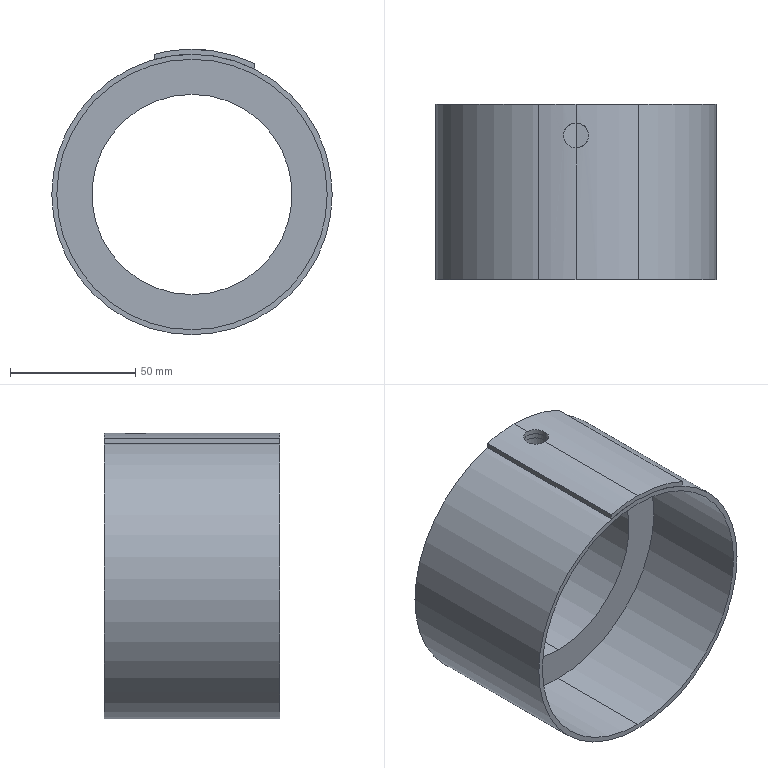Part | SolidWorks | features ICE 3, Extrusion 1 | 3 solids | 26 faces | box 112 x 70 x 114 mm | volume 156072 mm3 | cylinder 18 | plane 8 | commonest cylinder face diameters 10 x6 108 x4 112 x4 80 x2 116 x2
STEP:
#1=CARTESIAN_POINT('',(0.,7.5,54.));
#2=VERTEX_POINT('',#1);
#3=CARTESIAN_POINT('',(5.,12.5,53.768));
#4=VERTEX_POINT('',#3);
#5=CARTESIAN_POINT('',(0.,7.5,54.));
#6=CARTESIAN_POINT('',(0.3262,7.5,54.));
#7=CARTESIAN_POINT('',(0.6576,7.533,53.997));
#8=CARTESIAN_POINT('',(1.299,7.661,53.985));
#9=CARTESIAN_POINT('',(1.611,7.755,53.977));
#10=CARTESIAN_POINT('',(2.065,7.943,53.961));
#11=CARTESIAN_POINT('',(2.214,8.014,53.955));
#12=CARTESIAN_POINT('',(2.504,8.169,53.942));
#13=CARTESIAN_POINT('',(2.644,8.253,53.935));
#14=CARTESIAN_POINT('',(3.05,8.524,53.914));
#15=CARTESIAN_POINT('',(3.302,8.731,53.899));
#16=CARTESIAN_POINT('',(3.769,9.198,53.869));
#17=CARTESIAN_POINT('',(3.976,9.45,53.854));
#18=CARTESIAN_POINT('',(4.247,9.856,53.833));
#19=CARTESIAN_POINT('',(4.331,9.996,53.826));
#20=CARTESIAN_POINT('',(4.486,10.286,53.813));
#21=CARTESIAN_POINT('',(4.557,10.435,53.807));
#22=CARTESIAN_POINT('',(4.745,10.89,53.791));
#23=CARTESIAN_POINT('',(4.839,11.201,53.783));
#24=CARTESIAN_POINT('',(4.967,11.842,53.771));
#25=CARTESIAN_POINT('',(5.,12.174,53.768));
#26=CARTESIAN_POINT('',(5.,12.5,53.768));
#27=B_SPLINE_CURVE_WITH_KNOTS('',3,(#5,#6,#7,#8,#9,#10,#11,#12,#13,#14,#15,#16,#17,#18,#19,#20,#21,#22,#23,#24,#25,#26),.UNSPECIFIED.,.F.,.F.,(4,2,2,2,2,2,2,2,2,2,4),(0.007822,0.008799,0.009777,0.01027,0.01075,0.01173,0.01271,0.0132,0.01369,0.01466,0.01564),.UNSPECIFIED.);
#28=EDGE_CURVE('',#2,#4,#27,.T.);
#29=ORIENTED_EDGE('',*,*,#28,.T.);
#30=CARTESIAN_POINT('',(5.,12.5,39.686));
#31=VERTEX_POINT('',#30);
#32=CARTESIAN_POINT('',(5.,12.5,58.));
#33=DIRECTION('',(0.,0.,-1.));
#34=VECTOR('',#33,1000.);
#35=LINE('',#32,#34);
#36=EDGE_CURVE('',#4,#31,#35,.T.);
#37=ORIENTED_EDGE('',*,*,#36,.T.);
#38=CARTESIAN_POINT('',(0.,7.5,40.));
#39=VERTEX_POINT('',#38);
#40=CARTESIAN_POINT('',(0.,7.5,40.));
#41=CARTESIAN_POINT('',(0.3264,7.5,40.));
#42=CARTESIAN_POINT('',(0.658,7.533,39.996));
#43=CARTESIAN_POINT('',(1.299,7.661,39.98));
#44=CARTESIAN_POINT('',(1.611,7.755,39.969));
#45=CARTESIAN_POINT('',(2.065,7.944,39.947));
#46=CARTESIAN_POINT('',(2.215,8.014,39.939));
#47=CARTESIAN_POINT('',(2.504,8.169,39.922));
#48=CARTESIAN_POINT('',(2.644,8.253,39.913));
#49=CARTESIAN_POINT('',(3.05,8.525,39.884));
#50=CARTESIAN_POINT('',(3.303,8.732,39.864));
#51=CARTESIAN_POINT('',(3.769,9.198,39.823));
#52=CARTESIAN_POINT('',(3.976,9.45,39.802));
#53=CARTESIAN_POINT('',(4.247,9.856,39.774));
#54=CARTESIAN_POINT('',(4.331,9.996,39.765));
#55=CARTESIAN_POINT('',(4.486,10.285,39.748));
#56=CARTESIAN_POINT('',(4.557,10.435,39.74));
#57=CARTESIAN_POINT('',(4.745,10.889,39.718));
#58=CARTESIAN_POINT('',(4.839,11.201,39.706));
#59=CARTESIAN_POINT('',(4.967,11.842,39.69));
#60=CARTESIAN_POINT('',(5.,12.174,39.686));
#61=CARTESIAN_POINT('',(5.,12.5,39.686));
#62=B_SPLINE_CURVE_WITH_KNOTS('',3,(#40,#41,#42,#43,#44,#45,#46,#47,#48,#49,#50,#51,#52,#53,#54,#55,#56,#57,#58,#59,#60,#61),.UNSPECIFIED.,.F.,.F.,(4,2,2,2,2,2,2,2,2,2,4),(0.007826,0.008803,0.009781,0.01027,0.01076,0.01174,0.01271,0.0132,0.01369,0.01467,0.01565),.UNSPECIFIED.);
#63=EDGE_CURVE('',#39,#31,#62,.T.);
#64=ORIENTED_EDGE('',*,*,#63,.F.);
#65=CARTESIAN_POINT('',(-5.,12.5,39.686));
#66=VERTEX_POINT('',#65);
#67=CARTESIAN_POINT('',(-5.,12.5,39.686));
#68=CARTESIAN_POINT('',(-5.,12.169,39.686));
#69=CARTESIAN_POINT('',(-4.967,11.844,39.69));
#70=CARTESIAN_POINT('',(-4.872,11.364,39.702));
#71=CARTESIAN_POINT('',(-4.832,11.206,39.707));
#72=CARTESIAN_POINT('',(-4.737,10.891,39.719));
#73=CARTESIAN_POINT('',(-4.681,10.735,39.725));
#74=CARTESIAN_POINT('',(-4.493,10.281,39.747));
#75=CARTESIAN_POINT('',(-4.339,9.994,39.764));
#76=CARTESIAN_POINT('',(-3.976,9.45,39.802));
#77=CARTESIAN_POINT('',(-3.765,9.193,39.823));
#78=CARTESIAN_POINT('',(-3.304,8.733,39.864));
#79=CARTESIAN_POINT('',(-3.052,8.526,39.884));
#80=CARTESIAN_POINT('',(-2.505,8.16,39.922));
#81=CARTESIAN_POINT('',(-2.215,8.005,39.94));
#82=CARTESIAN_POINT('',(-1.613,7.756,39.969));
#83=CARTESIAN_POINT('',(-1.297,7.66,39.98));
#84=CARTESIAN_POINT('',(-0.6513,7.532,39.996));
#85=CARTESIAN_POINT('',(-0.3266,7.5,40.));
#86=CARTESIAN_POINT('',(0.,7.5,40.));
#87=B_SPLINE_CURVE_WITH_KNOTS('',3,(#67,#68,#69,#70,#71,#72,#73,#74,#75,#76,#77,#78,#79,#80,#81,#82,#83,#84,#85,#86),.UNSPECIFIED.,.F.,.F.,(4,2,2,2,2,2,2,2,2,4),(0.,0.0009782,0.001467,0.001956,0.002935,0.003913,0.004891,0.005869,0.006847,0.007826),.UNSPECIFIED.);
#88=EDGE_CURVE('',#66,#39,#87,.T.);
#89=ORIENTED_EDGE('',*,*,#88,.F.);
#90=CARTESIAN_POINT('',(-5.,12.5,53.768));
#91=VERTEX_POINT('',#90);
#92=CARTESIAN_POINT('',(-5.,12.5,58.));
#93=DIRECTION('',(0.,0.,-1.));
#94=VECTOR('',#93,1000.);
#95=LINE('',#92,#94);
#96=EDGE_CURVE('',#91,#66,#95,.T.);
#97=ORIENTED_EDGE('',*,*,#96,.F.);
#98=CARTESIAN_POINT('',(-5.,12.5,53.768));
#99=CARTESIAN_POINT('',(-5.,12.169,53.768));
#100=CARTESIAN_POINT('',(-4.968,11.844,53.771));
#101=CARTESIAN_POINT('',(-4.872,11.365,53.78));
#102=CARTESIAN_POINT('',(-4.832,11.206,53.783));
#103=CARTESIAN_POINT('',(-4.737,10.892,53.792));
#104=CARTESIAN_POINT('',(-4.681,10.736,53.797));
#105=CARTESIAN_POINT('',(-4.493,10.282,53.813));
#106=CARTESIAN_POINT('',(-4.339,9.994,53.826));
#107=CARTESIAN_POINT('',(-3.976,9.451,53.854));
#108=CARTESIAN_POINT('',(-3.765,9.194,53.869));
#109=CARTESIAN_POINT('',(-3.304,8.733,53.899));
#110=CARTESIAN_POINT('',(-3.052,8.526,53.914));
#111=CARTESIAN_POINT('',(-2.505,8.16,53.943));
#112=CARTESIAN_POINT('',(-2.214,8.005,53.955));
#113=CARTESIAN_POINT('',(-1.612,7.756,53.977));
#114=CARTESIAN_POINT('',(-1.297,7.66,53.985));
#115=CARTESIAN_POINT('',(-0.651,7.532,53.997));
#116=CARTESIAN_POINT('',(-0.3264,7.5,54.));
#117=CARTESIAN_POINT('',(0.,7.5,54.));
#118=B_SPLINE_CURVE_WITH_KNOTS('',3,(#98,#99,#100,#101,#102,#103,#104,#105,#106,#107,#108,#109,#110,#111,#112,#113,#114,#115,#116,#117),.UNSPECIFIED.,.F.,.F.,(4,2,2,2,2,2,2,2,2,4),(0.,0.0009778,0.001467,0.001956,0.002933,0.003911,0.004889,0.005867,0.006844,0.007822),.UNSPECIFIED.);
#119=EDGE_CURVE('',#91,#2,#118,.T.);
#120=ORIENTED_EDGE('',*,*,#119,.T.);
#121=EDGE_LOOP('',(#29,#37,#64,#89,#97,#120));
#122=FACE_OUTER_BOUND('',#121,.T.);
#123=CARTESIAN_POINT('',(0.,12.5,58.));
#124=DIRECTION('',(0.,0.,-1.));
#125=DIRECTION('',(-1.,0.,0.));
#126=AXIS2_PLACEMENT_3D('',#123,#124,#125);
#127=CYLINDRICAL_SURFACE('',#126,5.);
#128=ADVANCED_FACE('',(#122),#127,.F.);
#129=CARTESIAN_POINT('',(0.,25.,-40.));
#130=VERTEX_POINT('',#129);
#131=CARTESIAN_POINT('',(0.,25.,40.));
#132=VERTEX_POINT('',#131);
#133=CARTESIAN_POINT('',(0.,25.,0.));
#134=DIRECTION('',(0.,1.,0.));
#135=DIRECTION('',(0.,0.,1.));
#136=AXIS2_PLACEMENT_3D('',#133,#134,#135);
#137=CIRCLE('',#136,40.);
#138=EDGE_CURVE('',#130,#132,#137,.T.);
#139=ORIENTED_EDGE('',*,*,#138,.T.);
#140=CARTESIAN_POINT('',(0.,17.5,40.));
#141=VERTEX_POINT('',#140);
#142=CARTESIAN_POINT('',(0.,25.,40.));
#143=DIRECTION('',(0.,-1.,0.));
#144=VECTOR('',#143,1000.);
#145=LINE('',#142,#144);
#146=EDGE_CURVE('',#132,#141,#145,.T.);
#147=ORIENTED_EDGE('',*,*,#146,.T.);
#148=CARTESIAN_POINT('',(0.,17.5,40.));
#149=CARTESIAN_POINT('',(-0.3304,17.5,40.));
#150=CARTESIAN_POINT('',(-0.6553,17.468,39.996));
#151=CARTESIAN_POINT('',(-1.294,17.341,39.98));
#152=CARTESIAN_POINT('',(-1.612,17.244,39.969));
#153=CARTESIAN_POINT('',(-2.217,16.994,39.94));
#154=CARTESIAN_POINT('',(-2.504,16.84,39.922));
#155=CARTESIAN_POINT('',(-3.047,16.478,39.885));
#156=CARTESIAN_POINT('',(-3.304,16.267,39.864));
#157=CARTESIAN_POINT('',(-3.765,15.807,39.823));
#158=CARTESIAN_POINT('',(-3.972,15.555,39.803));
#159=CARTESIAN_POINT('',(-4.337,15.009,39.765));
#160=CARTESIAN_POINT('',(-4.492,14.719,39.747));
#161=CARTESIAN_POINT('',(-4.742,14.118,39.718));
#162=CARTESIAN_POINT('',(-4.838,13.803,39.706));
#163=CARTESIAN_POINT('',(-4.968,13.157,39.69));
#164=CARTESIAN_POINT('',(-5.,12.83,39.686));
#165=CARTESIAN_POINT('',(-5.,12.5,39.686));
#166=B_SPLINE_CURVE_WITH_KNOTS('',3,(#148,#149,#150,#151,#152,#153,#154,#155,#156,#157,#158,#159,#160,#161,#162,#163,#164,#165),.UNSPECIFIED.,.F.,.F.,(4,2,2,2,2,2,2,2,4),(0.02347,0.02445,0.02543,0.0264,0.02738,0.02836,0.02934,0.03031,0.03129),.UNSPECIFIED.);
#167=EDGE_CURVE('',#141,#66,#166,.T.);
#168=ORIENTED_EDGE('',*,*,#167,.T.);
#169=ORIENTED_EDGE('',*,*,#88,.T.);
#170=CARTESIAN_POINT('',(0.,0.,40.));
#171=VERTEX_POINT('',#170);
#172=CARTESIAN_POINT('',(0.,25.,40.));
#173=DIRECTION('',(0.,-1.,0.));
#174=VECTOR('',#173,1000.);
#175=LINE('',#172,#174);
#176=EDGE_CURVE('',#39,#171,#175,.T.);
#177=ORIENTED_EDGE('',*,*,#176,.T.);
#178=CARTESIAN_POINT('',(0.,0.,-40.));
#179=VERTEX_POINT('',#178);
#180=CARTESIAN_POINT('',(0.,0.,0.));
#181=DIRECTION('',(0.,1.,0.));
#182=DIRECTION('',(0.,0.,1.));
#183=AXIS2_PLACEMENT_3D('',#180,#181,#182);
#184=CIRCLE('',#183,40.);
#185=EDGE_CURVE('',#179,#171,#184,.T.);
#186=ORIENTED_EDGE('',*,*,#185,.F.);
#187=CARTESIAN_POINT('',(0.,25.,-40.));
#188=DIRECTION('',(0.,-1.,0.));
#189=VECTOR('',#188,1000.);
#190=LINE('',#187,#189);
#191=EDGE_CURVE('',#130,#179,#190,.T.);
#192=ORIENTED_EDGE('',*,*,#191,.F.);
#193=EDGE_LOOP('',(#139,#147,#168,#169,#177,#186,#192));
#194=FACE_OUTER_BOUND('',#193,.T.);
#195=CARTESIAN_POINT('',(0.,25.,0.));
#196=DIRECTION('',(0.,-1.,0.));
#197=DIRECTION('',(0.,0.,-1.));
#198=AXIS2_PLACEMENT_3D('',#195,#196,#197);
#199=CYLINDRICAL_SURFACE('',#198,40.);
#200=ADVANCED_FACE('',(#194),#199,.F.);
#201=CARTESIAN_POINT('',(0.,25.,54.));
#202=VERTEX_POINT('',#201);
#203=CARTESIAN_POINT('',(0.,25.,-54.));
#204=VERTEX_POINT('',#203);
#205=CARTESIAN_POINT('',(0.,25.,0.));
#206=DIRECTION('',(0.,1.,0.));
#207=DIRECTION('',(0.,0.,1.));
#208=AXIS2_PLACEMENT_3D('',#205,#206,#207);
#209=CIRCLE('',#208,54.);
#210=EDGE_CURVE('',#202,#204,#209,.T.);
#211=ORIENTED_EDGE('',*,*,#210,.F.);
#212=CARTESIAN_POINT('',(0.,17.5,54.));
#213=VERTEX_POINT('',#212);
#214=CARTESIAN_POINT('',(0.,25.,54.));
#215=DIRECTION('',(0.,-1.,0.));
#216=VECTOR('',#215,1000.);
#217=LINE('',#214,#216);
#218=EDGE_CURVE('',#202,#213,#217,.T.);
#219=ORIENTED_EDGE('',*,*,#218,.T.);
#220=CARTESIAN_POINT('',(5.,12.5,53.768));
#221=CARTESIAN_POINT('',(5.,12.826,53.768));
#222=CARTESIAN_POINT('',(4.968,13.151,53.771));
#223=CARTESIAN_POINT('',(4.84,13.796,53.783));
#224=CARTESIAN_POINT('',(4.744,14.112,53.791));
#225=CARTESIAN_POINT('',(4.495,14.714,53.813));
#226=CARTESIAN_POINT('',(4.34,15.005,53.826));
#227=CARTESIAN_POINT('',(3.974,15.552,53.854));
#228=CARTESIAN_POINT('',(3.767,15.804,53.869));
#229=CARTESIAN_POINT('',(3.306,16.265,53.899));
#230=CARTESIAN_POINT('',(3.049,16.476,53.915));
#231=CARTESIAN_POINT('',(2.505,16.839,53.943));
#232=CARTESIAN_POINT('',(2.218,16.993,53.955));
#233=CARTESIAN_POINT('',(1.764,17.181,53.971));
#234=CARTESIAN_POINT('',(1.608,17.237,53.976));
#235=CARTESIAN_POINT('',(1.294,17.333,53.985));
#236=CARTESIAN_POINT('',(1.135,17.372,53.988));
#237=CARTESIAN_POINT('',(0.6554,17.468,53.997));
#238=CARTESIAN_POINT('',(0.3304,17.5,54.));
#239=CARTESIAN_POINT('',(0.,17.5,54.));
#240=B_SPLINE_CURVE_WITH_KNOTS('',3,(#220,#221,#222,#223,#224,#225,#226,#227,#228,#229,#230,#231,#232,#233,#234,#235,#236,#237,#238,#239),.UNSPECIFIED.,.F.,.F.,(4,2,2,2,2,2,2,2,2,4),(0.01564,0.01662,0.0176,0.01857,0.01955,0.02053,0.02151,0.022,0.02249,0.02346),.UNSPECIFIED.);
#241=EDGE_CURVE('',#4,#213,#240,.T.);
#242=ORIENTED_EDGE('',*,*,#241,.F.);
#243=ORIENTED_EDGE('',*,*,#28,.F.);
#244=CARTESIAN_POINT('',(0.,0.,54.));
#245=VERTEX_POINT('',#244);
#246=CARTESIAN_POINT('',(0.,25.,54.));
#247=DIRECTION('',(0.,-1.,0.));
#248=VECTOR('',#247,1000.);
#249=LINE('',#246,#248);
#250=EDGE_CURVE('',#2,#245,#249,.T.);
#251=ORIENTED_EDGE('',*,*,#250,.T.);
#252=CARTESIAN_POINT('',(0.,0.,-54.));
#253=VERTEX_POINT('',#252);
#254=CARTESIAN_POINT('',(0.,0.,0.));
#255=DIRECTION('',(0.,1.,0.));
#256=DIRECTION('',(0.,0.,1.));
#257=AXIS2_PLACEMENT_3D('',#254,#255,#256);
#258=CIRCLE('',#257,54.);
#259=EDGE_CURVE('',#245,#253,#258,.T.);
#260=ORIENTED_EDGE('',*,*,#259,.T.);
#261=CARTESIAN_POINT('',(0.,25.,-54.));
#262=DIRECTION('',(0.,-1.,0.));
#263=VECTOR('',#262,1000.);
#264=LINE('',#261,#263);
#265=EDGE_CURVE('',#204,#253,#264,.T.);
#266=ORIENTED_EDGE('',*,*,#265,.F.);
#267=EDGE_LOOP('',(#211,#219,#242,#243,#251,#260,#266));
#268=FACE_OUTER_BOUND('',#267,.T.);
#269=CARTESIAN_POINT('',(0.,25.,0.));
#270=DIRECTION('',(0.,-1.,0.));
#271=DIRECTION('',(0.,0.,-1.));
#272=AXIS2_PLACEMENT_3D('',#269,#270,#271);
#273=CYLINDRICAL_SURFACE('',#272,54.);
#274=ADVANCED_FACE('',(#268),#273,.T.);
#275=ORIENTED_EDGE('',*,*,#218,.F.);
#276=CARTESIAN_POINT('',(0.,25.,0.));
#277=DIRECTION('',(0.,1.,0.));
#278=DIRECTION('',(0.,0.,1.));
#279=AXIS2_PLACEMENT_3D('',#276,#277,#278);
#280=CIRCLE('',#279,54.);
#281=EDGE_CURVE('',#204,#202,#280,.T.);
#282=ORIENTED_EDGE('',*,*,#281,.F.);
#283=ORIENTED_EDGE('',*,*,#265,.T.);
#284=CARTESIAN_POINT('',(0.,0.,0.));
#285=DIRECTION('',(0.,1.,0.));
#286=DIRECTION('',(0.,0.,1.));
#287=AXIS2_PLACEMENT_3D('',#284,#285,#286);
#288=CIRCLE('',#287,54.);
#289=EDGE_CURVE('',#253,#245,#288,.T.);
#290=ORIENTED_EDGE('',*,*,#289,.T.);
#291=ORIENTED_EDGE('',*,*,#250,.F.);
#292=ORIENTED_EDGE('',*,*,#119,.F.);
#293=CARTESIAN_POINT('',(0.,17.5,54.));
#294=CARTESIAN_POINT('',(-0.3301,17.5,54.));
#295=CARTESIAN_POINT('',(-0.6554,17.468,53.997));
#296=CARTESIAN_POINT('',(-1.135,17.372,53.988));
#297=CARTESIAN_POINT('',(-1.293,17.333,53.985));
#298=CARTESIAN_POINT('',(-1.607,17.238,53.976));
#299=CARTESIAN_POINT('',(-1.763,17.182,53.971));
#300=CARTESIAN_POINT('',(-2.217,16.994,53.955));
#301=CARTESIAN_POINT('',(-2.504,16.84,53.943));
#302=CARTESIAN_POINT('',(-3.047,16.478,53.915));
#303=CARTESIAN_POINT('',(-3.304,16.267,53.899));
#304=CARTESIAN_POINT('',(-3.765,15.806,53.869));
#305=CARTESIAN_POINT('',(-3.972,15.555,53.854));
#306=CARTESIAN_POINT('',(-4.337,15.009,53.826));
#307=CARTESIAN_POINT('',(-4.493,14.719,53.813));
#308=CARTESIAN_POINT('',(-4.742,14.117,53.792));
#309=CARTESIAN_POINT('',(-4.838,13.803,53.783));
#310=CARTESIAN_POINT('',(-4.968,13.157,53.771));
#311=CARTESIAN_POINT('',(-5.,12.83,53.768));
#312=CARTESIAN_POINT('',(-5.,12.5,53.768));
#313=B_SPLINE_CURVE_WITH_KNOTS('',3,(#293,#294,#295,#296,#297,#298,#299,#300,#301,#302,#303,#304,#305,#306,#307,#308,#309,#310,#311,#312),.UNSPECIFIED.,.F.,.F.,(4,2,2,2,2,2,2,2,2,4),(0.02346,0.02444,0.02493,0.02542,0.02639,0.02737,0.02835,0.02932,0.0303,0.03128),.UNSPECIFIED.);
#314=EDGE_CURVE('',#213,#91,#313,.T.);
#315=ORIENTED_EDGE('',*,*,#314,.F.);
#316=EDGE_LOOP('',(#275,#282,#283,#290,#291,#292,#315));
#317=FACE_OUTER_BOUND('',#316,.T.);
#318=CARTESIAN_POINT('',(0.,25.,0.));
#319=DIRECTION('',(0.,-1.,0.));
#320=DIRECTION('',(0.,0.,-1.));
#321=AXIS2_PLACEMENT_3D('',#318,#319,#320);
#322=CYLINDRICAL_SURFACE('',#321,54.);
#323=ADVANCED_FACE('',(#317),#322,.T.);
#324=ORIENTED_EDGE('',*,*,#146,.F.);
#325=CARTESIAN_POINT('',(0.,25.,0.));
#326=DIRECTION('',(0.,1.,0.));
#327=DIRECTION('',(0.,0.,1.));
#328=AXIS2_PLACEMENT_3D('',#325,#326,#327);
#329=CIRCLE('',#328,40.);
#330=EDGE_CURVE('',#132,#130,#329,.T.);
#331=ORIENTED_EDGE('',*,*,#330,.T.);
#332=ORIENTED_EDGE('',*,*,#191,.T.);
#333=CARTESIAN_POINT('',(0.,0.,0.));
#334=DIRECTION('',(0.,1.,0.));
#335=DIRECTION('',(0.,0.,1.));
#336=AXIS2_PLACEMENT_3D('',#333,#334,#335);
#337=CIRCLE('',#336,40.);
#338=EDGE_CURVE('',#171,#179,#337,.T.);
#339=ORIENTED_EDGE('',*,*,#338,.F.);
#340=ORIENTED_EDGE('',*,*,#176,.F.);
#341=ORIENTED_EDGE('',*,*,#63,.T.);
#342=CARTESIAN_POINT('',(5.,12.5,39.686));
#343=CARTESIAN_POINT('',(5.,12.827,39.686));
#344=CARTESIAN_POINT('',(4.968,13.151,39.69));
#345=CARTESIAN_POINT('',(4.84,13.797,39.706));
#346=CARTESIAN_POINT('',(4.744,14.113,39.718));
#347=CARTESIAN_POINT('',(4.495,14.715,39.747));
#348=CARTESIAN_POINT('',(4.339,15.006,39.764));
#349=CARTESIAN_POINT('',(3.974,15.552,39.803));
#350=CARTESIAN_POINT('',(3.767,15.804,39.823));
#351=CARTESIAN_POINT('',(3.306,16.265,39.864));
#352=CARTESIAN_POINT('',(3.049,16.476,39.885));
#353=CARTESIAN_POINT('',(2.506,16.839,39.922));
#354=CARTESIAN_POINT('',(2.219,16.993,39.94));
#355=CARTESIAN_POINT('',(1.765,17.181,39.961));
#356=CARTESIAN_POINT('',(1.608,17.237,39.968));
#357=CARTESIAN_POINT('',(1.294,17.332,39.979));
#358=CARTESIAN_POINT('',(1.136,17.372,39.984));
#359=CARTESIAN_POINT('',(0.6561,17.467,39.996));
#360=CARTESIAN_POINT('',(0.3307,17.5,40.));
#361=CARTESIAN_POINT('',(0.,17.5,40.));
#362=B_SPLINE_CURVE_WITH_KNOTS('',3,(#342,#343,#344,#345,#346,#347,#348,#349,#350,#351,#352,#353,#354,#355,#356,#357,#358,#359,#360,#361),.UNSPECIFIED.,.F.,.F.,(4,2,2,2,2,2,2,2,2,4),(0.01565,0.01663,0.0176,0.01858,0.01956,0.02054,0.02152,0.02201,0.02249,0.02347),.UNSPECIFIED.);
#363=EDGE_CURVE('',#31,#141,#362,.T.);
#364=ORIENTED_EDGE('',*,*,#363,.T.);
#365=EDGE_LOOP('',(#324,#331,#332,#339,#340,#341,#364));
#366=FACE_OUTER_BOUND('',#365,.T.);
#367=CARTESIAN_POINT('',(0.,25.,0.));
#368=DIRECTION('',(0.,-1.,0.));
#369=DIRECTION('',(0.,0.,-1.));
#370=AXIS2_PLACEMENT_3D('',#367,#368,#369);
#371=CYLINDRICAL_SURFACE('',#370,40.);
#372=ADVANCED_FACE('',(#366),#371,.F.);
#373=ORIENTED_EDGE('',*,*,#281,.T.);
#374=ORIENTED_EDGE('',*,*,#210,.T.);
#375=EDGE_LOOP('',(#373,#374));
#376=FACE_OUTER_BOUND('',#375,.T.);
#377=ORIENTED_EDGE('',*,*,#138,.F.);
#378=ORIENTED_EDGE('',*,*,#330,.F.);
#379=EDGE_LOOP('',(#377,#378));
#380=FACE_BOUND('',#379,.T.);
#381=CARTESIAN_POINT('',(0.,25.,0.));
#382=DIRECTION('',(0.,1.,0.));
#383=DIRECTION('',(0.,0.,1.));
#384=AXIS2_PLACEMENT_3D('',#381,#382,#383);
#385=PLANE('',#384);
#386=ADVANCED_FACE('',(#376,#380),#385,.T.);
#387=ORIENTED_EDGE('',*,*,#289,.F.);
#388=ORIENTED_EDGE('',*,*,#259,.F.);
#389=EDGE_LOOP('',(#387,#388));
#390=FACE_OUTER_BOUND('',#389,.T.);
#391=ORIENTED_EDGE('',*,*,#185,.T.);
#392=ORIENTED_EDGE('',*,*,#338,.T.);
#393=EDGE_LOOP('',(#391,#392));
#394=FACE_BOUND('',#393,.T.);
#395=CARTESIAN_POINT('',(0.,0.,0.));
#396=DIRECTION('',(0.,1.,0.));
#397=DIRECTION('',(0.,0.,1.));
#398=AXIS2_PLACEMENT_3D('',#395,#396,#397);
#399=PLANE('',#398);
#400=ADVANCED_FACE('',(#390,#394),#399,.F.);
#401=ORIENTED_EDGE('',*,*,#36,.F.);
#402=ORIENTED_EDGE('',*,*,#241,.T.);
#403=ORIENTED_EDGE('',*,*,#314,.T.);
#404=ORIENTED_EDGE('',*,*,#96,.T.);
#405=ORIENTED_EDGE('',*,*,#167,.F.);
#406=ORIENTED_EDGE('',*,*,#363,.F.);
#407=EDGE_LOOP('',(#401,#402,#403,#404,#405,#406));
#408=FACE_OUTER_BOUND('',#407,.T.);
#409=CARTESIAN_POINT('',(0.,12.5,58.));
#410=DIRECTION('',(0.,0.,-1.));
#411=DIRECTION('',(-1.,0.,0.));
#412=AXIS2_PLACEMENT_3D('',#409,#410,#411);
#413=CYLINDRICAL_SURFACE('',#412,5.);
#414=ADVANCED_FACE('',(#408),#413,.F.);
#415=CLOSED_SHELL('',(#128,#200,#274,#323,#372,#386,#400,#414));
#416=MANIFOLD_SOLID_BREP('',#415);
#417=CARTESIAN_POINT('',(5.,12.5,55.776));
#418=VERTEX_POINT('',#417);
#419=CARTESIAN_POINT('',(0.,7.5,56.));
#420=VERTEX_POINT('',#419);
#421=CARTESIAN_POINT('',(5.,12.5,55.776));
#422=CARTESIAN_POINT('',(5.,12.17,55.776));
#423=CARTESIAN_POINT('',(4.968,11.845,55.779));
#424=CARTESIAN_POINT('',(4.872,11.366,55.788));
#425=CARTESIAN_POINT('',(4.833,11.207,55.791));
#426=CARTESIAN_POINT('',(4.738,10.893,55.799));
#427=CARTESIAN_POINT('',(4.682,10.737,55.804));
#428=CARTESIAN_POINT('',(4.494,10.283,55.82));
#429=CARTESIAN_POINT('',(4.34,9.996,55.832));
#430=CARTESIAN_POINT('',(3.978,9.453,55.859));
#431=CARTESIAN_POINT('',(3.767,9.196,55.874));
#432=CARTESIAN_POINT('',(3.306,8.735,55.903));
#433=CARTESIAN_POINT('',(3.055,8.528,55.917));
#434=CARTESIAN_POINT('',(2.509,8.163,55.944));
#435=CARTESIAN_POINT('',(2.218,8.007,55.957));
#436=CARTESIAN_POINT('',(1.617,7.758,55.977));
#437=CARTESIAN_POINT('',(1.303,7.662,55.986));
#438=CARTESIAN_POINT('',(0.657,7.532,55.997));
#439=CARTESIAN_POINT('',(0.3303,7.5,56.));
#440=CARTESIAN_POINT('',(0.,7.5,56.));
#441=B_SPLINE_CURVE_WITH_KNOTS('',3,(#421,#422,#423,#424,#425,#426,#427,#428,#429,#430,#431,#432,#433,#434,#435,#436,#437,#438,#439,#440),.UNSPECIFIED.,.F.,.F.,(4,2,2,2,2,2,2,2,2,4),(0.02346,0.02444,0.02493,0.02542,0.02639,0.02737,0.02835,0.02932,0.0303,0.03128),.UNSPECIFIED.);
#442=EDGE_CURVE('',#418,#420,#441,.T.);
#443=ORIENTED_EDGE('',*,*,#442,.F.);
#444=CARTESIAN_POINT('',(5.,12.5,53.768));
#445=VERTEX_POINT('',#444);
#446=CARTESIAN_POINT('',(5.,12.5,58.));
#447=DIRECTION('',(0.,0.,-1.));
#448=VECTOR('',#447,1000.);
#449=LINE('',#446,#448);
#450=EDGE_CURVE('',#418,#445,#449,.T.);
#451=ORIENTED_EDGE('',*,*,#450,.T.);
#452=CARTESIAN_POINT('',(0.,7.5,54.));
#453=VERTEX_POINT('',#452);
#454=CARTESIAN_POINT('',(5.,12.5,53.768));
#455=CARTESIAN_POINT('',(5.,12.17,53.768));
#456=CARTESIAN_POINT('',(4.968,11.845,53.771));
#457=CARTESIAN_POINT('',(4.872,11.365,53.78));
#458=CARTESIAN_POINT('',(4.833,11.207,53.783));
#459=CARTESIAN_POINT('',(4.738,10.893,53.792));
#460=CARTESIAN_POINT('',(4.682,10.737,53.797));
#461=CARTESIAN_POINT('',(4.494,10.283,53.813));
#462=CARTESIAN_POINT('',(4.34,9.996,53.826));
#463=CARTESIAN_POINT('',(3.978,9.453,53.854));
#464=CARTESIAN_POINT('',(3.767,9.196,53.869));
#465=CARTESIAN_POINT('',(3.306,8.735,53.899));
#466=CARTESIAN_POINT('',(3.055,8.528,53.914));
#467=CARTESIAN_POINT('',(2.509,8.163,53.942));
#468=CARTESIAN_POINT('',(2.219,8.007,53.955));
#469=CARTESIAN_POINT('',(1.617,7.758,53.977));
#470=CARTESIAN_POINT('',(1.303,7.662,53.985));
#471=CARTESIAN_POINT('',(0.657,7.532,53.997));
#472=CARTESIAN_POINT('',(0.3303,7.5,54.));
#473=CARTESIAN_POINT('',(0.,7.5,54.));
#474=B_SPLINE_CURVE_WITH_KNOTS('',3,(#454,#455,#456,#457,#458,#459,#460,#461,#462,#463,#464,#465,#466,#467,#468,#469,#470,#471,#472,#473),.UNSPECIFIED.,.F.,.F.,(4,2,2,2,2,2,2,2,2,4),(0.02346,0.02444,0.02493,0.02542,0.02639,0.02737,0.02835,0.02932,0.0303,0.03128),.UNSPECIFIED.);
#475=EDGE_CURVE('',#445,#453,#474,.T.);
#476=ORIENTED_EDGE('',*,*,#475,.T.);
#477=CARTESIAN_POINT('',(-5.,12.5,53.768));
#478=VERTEX_POINT('',#477);
#479=CARTESIAN_POINT('',(0.,7.5,54.));
#480=CARTESIAN_POINT('',(-0.3306,7.5,54.));
#481=CARTESIAN_POINT('',(-0.6557,7.532,53.997));
#482=CARTESIAN_POINT('',(-1.135,7.628,53.988));
#483=CARTESIAN_POINT('',(-1.294,7.668,53.985));
#484=CARTESIAN_POINT('',(-1.608,7.763,53.976));
#485=CARTESIAN_POINT('',(-1.764,7.819,53.971));
#486=CARTESIAN_POINT('',(-2.218,8.007,53.955));
#487=CARTESIAN_POINT('',(-2.506,8.161,53.943));
#488=CARTESIAN_POINT('',(-3.049,8.524,53.915));
#489=CARTESIAN_POINT('',(-3.306,8.735,53.899));
#490=CARTESIAN_POINT('',(-3.767,9.196,53.869));
#491=CARTESIAN_POINT('',(-3.974,9.448,53.854));
#492=CARTESIAN_POINT('',(-4.34,9.995,53.826));
#493=CARTESIAN_POINT('',(-4.495,10.286,53.813));
#494=CARTESIAN_POINT('',(-4.744,10.888,53.791));
#495=CARTESIAN_POINT('',(-4.84,11.203,53.783));
#496=CARTESIAN_POINT('',(-4.968,11.849,53.771));
#497=CARTESIAN_POINT('',(-5.,12.174,53.768));
#498=CARTESIAN_POINT('',(-5.,12.5,53.768));
#499=B_SPLINE_CURVE_WITH_KNOTS('',3,(#479,#480,#481,#482,#483,#484,#485,#486,#487,#488,#489,#490,#491,#492,#493,#494,#495,#496,#497,#498),.UNSPECIFIED.,.F.,.F.,(4,2,2,2,2,2,2,2,2,4),(0.,0.0009778,0.001467,0.001956,0.002933,0.003911,0.004889,0.005867,0.006844,0.007822),.UNSPECIFIED.);
#500=EDGE_CURVE('',#453,#478,#499,.T.);
#501=ORIENTED_EDGE('',*,*,#500,.T.);
#502=CARTESIAN_POINT('',(-5.,12.5,55.776));
#503=VERTEX_POINT('',#502);
#504=CARTESIAN_POINT('',(-5.,12.5,58.));
#505=DIRECTION('',(0.,0.,-1.));
#506=VECTOR('',#505,1000.);
#507=LINE('',#504,#506);
#508=EDGE_CURVE('',#503,#478,#507,.T.);
#509=ORIENTED_EDGE('',*,*,#508,.F.);
#510=CARTESIAN_POINT('',(0.,7.5,56.));
#511=CARTESIAN_POINT('',(-0.3306,7.5,56.));
#512=CARTESIAN_POINT('',(-0.6557,7.532,55.997));
#513=CARTESIAN_POINT('',(-1.135,7.628,55.989));
#514=CARTESIAN_POINT('',(-1.294,7.667,55.985));
#515=CARTESIAN_POINT('',(-1.608,7.763,55.977));
#516=CARTESIAN_POINT('',(-1.764,7.819,55.972));
#517=CARTESIAN_POINT('',(-2.218,8.007,55.957));
#518=CARTESIAN_POINT('',(-2.506,8.161,55.945));
#519=CARTESIAN_POINT('',(-3.049,8.524,55.918));
#520=CARTESIAN_POINT('',(-3.306,8.735,55.903));
#521=CARTESIAN_POINT('',(-3.767,9.196,55.874));
#522=CARTESIAN_POINT('',(-3.974,9.448,55.859));
#523=CARTESIAN_POINT('',(-4.34,9.995,55.832));
#524=CARTESIAN_POINT('',(-4.495,10.286,55.819));
#525=CARTESIAN_POINT('',(-4.744,10.888,55.799));
#526=CARTESIAN_POINT('',(-4.84,11.203,55.79));
#527=CARTESIAN_POINT('',(-4.968,11.849,55.779));
#528=CARTESIAN_POINT('',(-5.,12.174,55.776));
#529=CARTESIAN_POINT('',(-5.,12.5,55.776));
#530=B_SPLINE_CURVE_WITH_KNOTS('',3,(#510,#511,#512,#513,#514,#515,#516,#517,#518,#519,#520,#521,#522,#523,#524,#525,#526,#527,#528,#529),.UNSPECIFIED.,.F.,.F.,(4,2,2,2,2,2,2,2,2,4),(0.,0.0009777,0.001467,0.001955,0.002933,0.003911,0.004889,0.005866,0.006844,0.007822),.UNSPECIFIED.);
#531=EDGE_CURVE('',#420,#503,#530,.T.);
#532=ORIENTED_EDGE('',*,*,#531,.F.);
#533=EDGE_LOOP('',(#443,#451,#476,#501,#509,#532));
#534=FACE_OUTER_BOUND('',#533,.T.);
#535=CARTESIAN_POINT('',(0.,12.5,58.));
#536=DIRECTION('',(0.,0.,-1.));
#537=DIRECTION('',(-1.,0.,0.));
#538=AXIS2_PLACEMENT_3D('',#535,#536,#537);
#539=CYLINDRICAL_SURFACE('',#538,5.);
#540=ADVANCED_FACE('',(#534),#539,.F.);
#541=CARTESIAN_POINT('',(0.,-45.,-54.));
#542=VERTEX_POINT('',#541);
#543=CARTESIAN_POINT('',(0.,-45.,54.));
#544=VERTEX_POINT('',#543);
#545=CARTESIAN_POINT('',(0.,-45.,0.));
#546=DIRECTION('',(0.,1.,0.));
#547=DIRECTION('',(0.,0.,1.));
#548=AXIS2_PLACEMENT_3D('',#545,#546,#547);
#549=CIRCLE('',#548,54.);
#550=EDGE_CURVE('',#542,#544,#549,.T.);
#551=ORIENTED_EDGE('',*,*,#550,.F.);
#552=CARTESIAN_POINT('',(0.,25.,-54.));
#553=VERTEX_POINT('',#552);
#554=CARTESIAN_POINT('',(0.,-45.,-54.));
#555=DIRECTION('',(0.,1.,0.));
#556=VECTOR('',#555,1000.);
#557=LINE('',#554,#556);
#558=EDGE_CURVE('',#542,#553,#557,.T.);
#559=ORIENTED_EDGE('',*,*,#558,.T.);
#560=CARTESIAN_POINT('',(0.,25.,54.));
#561=VERTEX_POINT('',#560);
#562=CARTESIAN_POINT('',(0.,25.,0.));
#563=DIRECTION('',(0.,1.,0.));
#564=DIRECTION('',(0.,0.,1.));
#565=AXIS2_PLACEMENT_3D('',#562,#563,#564);
#566=CIRCLE('',#565,54.);
#567=EDGE_CURVE('',#553,#561,#566,.T.);
#568=ORIENTED_EDGE('',*,*,#567,.T.);
#569=CARTESIAN_POINT('',(0.,17.5,54.));
#570=VERTEX_POINT('',#569);
#571=CARTESIAN_POINT('',(0.,-45.,54.));
#572=DIRECTION('',(0.,1.,0.));
#573=VECTOR('',#572,1000.);
#574=LINE('',#571,#573);
#575=EDGE_CURVE('',#570,#561,#574,.T.);
#576=ORIENTED_EDGE('',*,*,#575,.F.);
#577=CARTESIAN_POINT('',(-5.,12.5,53.768));
#578=CARTESIAN_POINT('',(-5.,12.826,53.768));
#579=CARTESIAN_POINT('',(-4.967,13.158,53.771));
#580=CARTESIAN_POINT('',(-4.839,13.799,53.783));
#581=CARTESIAN_POINT('',(-4.745,14.111,53.791));
#582=CARTESIAN_POINT('',(-4.557,14.565,53.807));
#583=CARTESIAN_POINT('',(-4.486,14.714,53.813));
#584=CARTESIAN_POINT('',(-4.331,15.004,53.826));
#585=CARTESIAN_POINT('',(-4.247,15.144,53.833));
#586=CARTESIAN_POINT('',(-3.976,15.55,53.854));
#587=CARTESIAN_POINT('',(-3.769,15.802,53.869));
#588=CARTESIAN_POINT('',(-3.302,16.269,53.899));
#589=CARTESIAN_POINT('',(-3.05,16.476,53.915));
#590=CARTESIAN_POINT('',(-2.644,16.747,53.935));
#591=CARTESIAN_POINT('',(-2.504,16.831,53.942));
#592=CARTESIAN_POINT('',(-2.214,16.986,53.955));
#593=CARTESIAN_POINT('',(-2.065,17.057,53.961));
#594=CARTESIAN_POINT('',(-1.61,17.245,53.977));
#595=CARTESIAN_POINT('',(-1.299,17.339,53.985));
#596=CARTESIAN_POINT('',(-0.6578,17.467,53.997));
#597=CARTESIAN_POINT('',(-0.3263,17.5,54.));
#598=CARTESIAN_POINT('',(0.,17.5,54.));
#599=B_SPLINE_CURVE_WITH_KNOTS('',3,(#577,#578,#579,#580,#581,#582,#583,#584,#585,#586,#587,#588,#589,#590,#591,#592,#593,#594,#595,#596,#597,#598),.UNSPECIFIED.,.F.,.F.,(4,2,2,2,2,2,2,2,2,2,4),(0.007822,0.008799,0.009777,0.01027,0.01075,0.01173,0.01271,0.0132,0.01369,0.01466,0.01564),.UNSPECIFIED.);
#600=EDGE_CURVE('',#478,#570,#599,.T.);
#601=ORIENTED_EDGE('',*,*,#600,.F.);
#602=ORIENTED_EDGE('',*,*,#500,.F.);
#603=CARTESIAN_POINT('',(0.,-45.,54.));
#604=DIRECTION('',(0.,1.,0.));
#605=VECTOR('',#604,1000.);
#606=LINE('',#603,#605);
#607=EDGE_CURVE('',#544,#453,#606,.T.);
#608=ORIENTED_EDGE('',*,*,#607,.F.);
#609=EDGE_LOOP('',(#551,#559,#568,#576,#601,#602,#608));
#610=FACE_OUTER_BOUND('',#609,.T.);
#611=CARTESIAN_POINT('',(0.,-45.,0.));
#612=DIRECTION('',(0.,1.,0.));
#613=DIRECTION('',(0.,0.,1.));
#614=AXIS2_PLACEMENT_3D('',#611,#612,#613);
#615=CYLINDRICAL_SURFACE('',#614,54.);
#616=ADVANCED_FACE('',(#610),#615,.F.);
#617=CARTESIAN_POINT('',(0.,-45.,56.));
#618=VERTEX_POINT('',#617);
#619=CARTESIAN_POINT('',(0.,-45.,-56.));
#620=VERTEX_POINT('',#619);
#621=CARTESIAN_POINT('',(0.,-45.,0.));
#622=DIRECTION('',(0.,1.,0.));
#623=DIRECTION('',(0.,0.,1.));
#624=AXIS2_PLACEMENT_3D('',#621,#622,#623);
#625=CIRCLE('',#624,56.);
#626=EDGE_CURVE('',#618,#620,#625,.T.);
#627=ORIENTED_EDGE('',*,*,#626,.T.);
#628=CARTESIAN_POINT('',(0.,25.,-56.));
#629=VERTEX_POINT('',#628);
#630=CARTESIAN_POINT('',(0.,-45.,-56.));
#631=DIRECTION('',(0.,1.,0.));
#632=VECTOR('',#631,1000.);
#633=LINE('',#630,#632);
#634=EDGE_CURVE('',#620,#629,#633,.T.);
#635=ORIENTED_EDGE('',*,*,#634,.T.);
#636=CARTESIAN_POINT('',(0.,25.,56.));
#637=VERTEX_POINT('',#636);
#638=CARTESIAN_POINT('',(0.,25.,0.));
#639=DIRECTION('',(0.,1.,0.));
#640=DIRECTION('',(0.,0.,1.));
#641=AXIS2_PLACEMENT_3D('',#638,#639,#640);
#642=CIRCLE('',#641,56.);
#643=EDGE_CURVE('',#637,#629,#642,.T.);
#644=ORIENTED_EDGE('',*,*,#643,.F.);
#645=CARTESIAN_POINT('',(0.,17.5,56.));
#646=VERTEX_POINT('',#645);
#647=CARTESIAN_POINT('',(0.,-45.,56.));
#648=DIRECTION('',(0.,1.,0.));
#649=VECTOR('',#648,1000.);
#650=LINE('',#647,#649);
#651=EDGE_CURVE('',#646,#637,#650,.T.);
#652=ORIENTED_EDGE('',*,*,#651,.F.);
#653=CARTESIAN_POINT('',(0.,17.5,56.));
#654=CARTESIAN_POINT('',(0.3265,17.5,56.));
#655=CARTESIAN_POINT('',(0.6511,17.468,55.997));
#656=CARTESIAN_POINT('',(1.296,17.34,55.986));
#657=CARTESIAN_POINT('',(1.612,17.244,55.978));
#658=CARTESIAN_POINT('',(2.214,16.995,55.957));
#659=CARTESIAN_POINT('',(2.505,16.84,55.945));
#660=CARTESIAN_POINT('',(3.052,16.474,55.917));
#661=CARTESIAN_POINT('',(3.304,16.267,55.903));
#662=CARTESIAN_POINT('',(3.765,15.806,55.874));
#663=CARTESIAN_POINT('',(3.976,15.549,55.859));
#664=CARTESIAN_POINT('',(4.339,15.005,55.832));
#665=CARTESIAN_POINT('',(4.493,14.718,55.82));
#666=CARTESIAN_POINT('',(4.744,14.113,55.799));
#667=CARTESIAN_POINT('',(4.84,13.795,55.79));
#668=CARTESIAN_POINT('',(4.968,13.155,55.779));
#669=CARTESIAN_POINT('',(5.,12.83,55.776));
#670=CARTESIAN_POINT('',(5.,12.5,55.776));
#671=B_SPLINE_CURVE_WITH_KNOTS('',3,(#653,#654,#655,#656,#657,#658,#659,#660,#661,#662,#663,#664,#665,#666,#667,#668,#669,#670),.UNSPECIFIED.,.F.,.F.,(4,2,2,2,2,2,2,2,4),(0.01564,0.01662,0.0176,0.01857,0.01955,0.02053,0.02151,0.02248,0.02346),.UNSPECIFIED.);
#672=EDGE_CURVE('',#646,#418,#671,.T.);
#673=ORIENTED_EDGE('',*,*,#672,.T.);
#674=ORIENTED_EDGE('',*,*,#442,.T.);
#675=CARTESIAN_POINT('',(0.,-45.,56.));
#676=DIRECTION('',(0.,1.,0.));
#677=VECTOR('',#676,1000.);
#678=LINE('',#675,#677);
#679=EDGE_CURVE('',#618,#420,#678,.T.);
#680=ORIENTED_EDGE('',*,*,#679,.F.);
#681=EDGE_LOOP('',(#627,#635,#644,#652,#673,#674,#680));
#682=FACE_OUTER_BOUND('',#681,.T.);
#683=CARTESIAN_POINT('',(0.,-45.,0.));
#684=DIRECTION('',(0.,1.,0.));
#685=DIRECTION('',(0.,0.,1.));
#686=AXIS2_PLACEMENT_3D('',#683,#684,#685);
#687=CYLINDRICAL_SURFACE('',#686,56.);
#688=ADVANCED_FACE('',(#682),#687,.T.);
#689=ORIENTED_EDGE('',*,*,#634,.F.);
#690=CARTESIAN_POINT('',(0.,-45.,0.));
#691=DIRECTION('',(0.,1.,0.));
#692=DIRECTION('',(0.,0.,1.));
#693=AXIS2_PLACEMENT_3D('',#690,#691,#692);
#694=CIRCLE('',#693,56.);
#695=EDGE_CURVE('',#620,#618,#694,.T.);
#696=ORIENTED_EDGE('',*,*,#695,.T.);
#697=ORIENTED_EDGE('',*,*,#679,.T.);
#698=ORIENTED_EDGE('',*,*,#531,.T.);
#699=CARTESIAN_POINT('',(-5.,12.5,55.776));
#700=CARTESIAN_POINT('',(-5.,12.826,55.776));
#701=CARTESIAN_POINT('',(-4.967,13.158,55.779));
#702=CARTESIAN_POINT('',(-4.839,13.799,55.791));
#703=CARTESIAN_POINT('',(-4.745,14.11,55.799));
#704=CARTESIAN_POINT('',(-4.557,14.565,55.814));
#705=CARTESIAN_POINT('',(-4.486,14.714,55.82));
#706=CARTESIAN_POINT('',(-4.331,15.004,55.832));
#707=CARTESIAN_POINT('',(-4.247,15.144,55.839));
#708=CARTESIAN_POINT('',(-3.976,15.55,55.859));
#709=CARTESIAN_POINT('',(-3.769,15.802,55.874));
#710=CARTESIAN_POINT('',(-3.302,16.269,55.903));
#711=CARTESIAN_POINT('',(-3.05,16.476,55.918));
#712=CARTESIAN_POINT('',(-2.644,16.747,55.938));
#713=CARTESIAN_POINT('',(-2.504,16.831,55.944));
#714=CARTESIAN_POINT('',(-2.214,16.986,55.956));
#715=CARTESIAN_POINT('',(-2.065,17.057,55.962));
#716=CARTESIAN_POINT('',(-1.61,17.245,55.978));
#717=CARTESIAN_POINT('',(-1.299,17.339,55.986));
#718=CARTESIAN_POINT('',(-0.6578,17.467,55.997));
#719=CARTESIAN_POINT('',(-0.3263,17.5,56.));
#720=CARTESIAN_POINT('',(0.,17.5,56.));
#721=B_SPLINE_CURVE_WITH_KNOTS('',3,(#699,#700,#701,#702,#703,#704,#705,#706,#707,#708,#709,#710,#711,#712,#713,#714,#715,#716,#717,#718,#719,#720),.UNSPECIFIED.,.F.,.F.,(4,2,2,2,2,2,2,2,2,2,4),(0.007822,0.008799,0.009776,0.01027,0.01075,0.01173,0.01271,0.0132,0.01369,0.01466,0.01564),.UNSPECIFIED.);
#722=EDGE_CURVE('',#503,#646,#721,.T.);
#723=ORIENTED_EDGE('',*,*,#722,.T.);
#724=ORIENTED_EDGE('',*,*,#651,.T.);
#725=CARTESIAN_POINT('',(0.,25.,0.));
#726=DIRECTION('',(0.,1.,0.));
#727=DIRECTION('',(0.,0.,1.));
#728=AXIS2_PLACEMENT_3D('',#725,#726,#727);
#729=CIRCLE('',#728,56.);
#730=EDGE_CURVE('',#629,#637,#729,.T.);
#731=ORIENTED_EDGE('',*,*,#730,.F.);
#732=EDGE_LOOP('',(#689,#696,#697,#698,#723,#724,#731));
#733=FACE_OUTER_BOUND('',#732,.T.);
#734=CARTESIAN_POINT('',(0.,-45.,0.));
#735=DIRECTION('',(0.,1.,0.));
#736=DIRECTION('',(0.,0.,1.));
#737=AXIS2_PLACEMENT_3D('',#734,#735,#736);
#738=CYLINDRICAL_SURFACE('',#737,56.);
#739=ADVANCED_FACE('',(#733),#738,.T.);
#740=ORIENTED_EDGE('',*,*,#558,.F.);
#741=CARTESIAN_POINT('',(0.,-45.,0.));
#742=DIRECTION('',(0.,1.,0.));
#743=DIRECTION('',(0.,0.,1.));
#744=AXIS2_PLACEMENT_3D('',#741,#742,#743);
#745=CIRCLE('',#744,54.);
#746=EDGE_CURVE('',#544,#542,#745,.T.);
#747=ORIENTED_EDGE('',*,*,#746,.F.);
#748=ORIENTED_EDGE('',*,*,#607,.T.);
#749=ORIENTED_EDGE('',*,*,#475,.F.);
#750=CARTESIAN_POINT('',(0.,17.5,54.));
#751=CARTESIAN_POINT('',(0.3265,17.5,54.));
#752=CARTESIAN_POINT('',(0.6511,17.468,53.997));
#753=CARTESIAN_POINT('',(1.296,17.34,53.985));
#754=CARTESIAN_POINT('',(1.612,17.244,53.977));
#755=CARTESIAN_POINT('',(2.214,16.995,53.955));
#756=CARTESIAN_POINT('',(2.505,16.84,53.943));
#757=CARTESIAN_POINT('',(3.052,16.474,53.914));
#758=CARTESIAN_POINT('',(3.304,16.267,53.899));
#759=CARTESIAN_POINT('',(3.765,15.806,53.869));
#760=CARTESIAN_POINT('',(3.976,15.549,53.854));
#761=CARTESIAN_POINT('',(4.339,15.005,53.826));
#762=CARTESIAN_POINT('',(4.493,14.718,53.813));
#763=CARTESIAN_POINT('',(4.681,14.264,53.797));
#764=CARTESIAN_POINT('',(4.737,14.108,53.792));
#765=CARTESIAN_POINT('',(4.833,13.794,53.783));
#766=CARTESIAN_POINT('',(4.872,13.635,53.78));
#767=CARTESIAN_POINT('',(4.968,13.155,53.771));
#768=CARTESIAN_POINT('',(5.,12.83,53.768));
#769=CARTESIAN_POINT('',(5.,12.5,53.768));
#770=B_SPLINE_CURVE_WITH_KNOTS('',3,(#750,#751,#752,#753,#754,#755,#756,#757,#758,#759,#760,#761,#762,#763,#764,#765,#766,#767,#768,#769),.UNSPECIFIED.,.F.,.F.,(4,2,2,2,2,2,2,2,2,4),(0.01564,0.01662,0.0176,0.01857,0.01955,0.02053,0.02151,0.022,0.02249,0.02346),.UNSPECIFIED.);
#771=EDGE_CURVE('',#570,#445,#770,.T.);
#772=ORIENTED_EDGE('',*,*,#771,.F.);
#773=ORIENTED_EDGE('',*,*,#575,.T.);
#774=CARTESIAN_POINT('',(0.,25.,0.));
#775=DIRECTION('',(0.,1.,0.));
#776=DIRECTION('',(0.,0.,1.));
#777=AXIS2_PLACEMENT_3D('',#774,#775,#776);
#778=CIRCLE('',#777,54.);
#779=EDGE_CURVE('',#561,#553,#778,.T.);
#780=ORIENTED_EDGE('',*,*,#779,.T.);
#781=EDGE_LOOP('',(#740,#747,#748,#749,#772,#773,#780));
#782=FACE_OUTER_BOUND('',#781,.T.);
#783=CARTESIAN_POINT('',(0.,-45.,0.));
#784=DIRECTION('',(0.,1.,0.));
#785=DIRECTION('',(0.,0.,1.));
#786=AXIS2_PLACEMENT_3D('',#783,#784,#785);
#787=CYLINDRICAL_SURFACE('',#786,54.);
#788=ADVANCED_FACE('',(#782),#787,.F.);
#789=ORIENTED_EDGE('',*,*,#746,.T.);
#790=ORIENTED_EDGE('',*,*,#550,.T.);
#791=EDGE_LOOP('',(#789,#790));
#792=FACE_BOUND('',#791,.T.);
#793=ORIENTED_EDGE('',*,*,#626,.F.);
#794=ORIENTED_EDGE('',*,*,#695,.F.);
#795=EDGE_LOOP('',(#793,#794));
#796=FACE_OUTER_BOUND('',#795,.T.);
#797=CARTESIAN_POINT('',(0.,-45.,0.));
#798=DIRECTION('',(0.,1.,0.));
#799=DIRECTION('',(0.,0.,1.));
#800=AXIS2_PLACEMENT_3D('',#797,#798,#799);
#801=PLANE('',#800);
#802=ADVANCED_FACE('',(#792,#796),#801,.F.);
#803=ORIENTED_EDGE('',*,*,#779,.F.);
#804=ORIENTED_EDGE('',*,*,#567,.F.);
#805=EDGE_LOOP('',(#803,#804));
#806=FACE_BOUND('',#805,.T.);
#807=ORIENTED_EDGE('',*,*,#643,.T.);
#808=ORIENTED_EDGE('',*,*,#730,.T.);
#809=EDGE_LOOP('',(#807,#808));
#810=FACE_OUTER_BOUND('',#809,.T.);
#811=CARTESIAN_POINT('',(0.,25.,0.));
#812=DIRECTION('',(0.,1.,0.));
#813=DIRECTION('',(0.,0.,1.));
#814=AXIS2_PLACEMENT_3D('',#811,#812,#813);
#815=PLANE('',#814);
#816=ADVANCED_FACE('',(#806,#810),#815,.T.);
#817=ORIENTED_EDGE('',*,*,#450,.F.);
#818=ORIENTED_EDGE('',*,*,#672,.F.);
#819=ORIENTED_EDGE('',*,*,#722,.F.);
#820=ORIENTED_EDGE('',*,*,#508,.T.);
#821=ORIENTED_EDGE('',*,*,#600,.T.);
#822=ORIENTED_EDGE('',*,*,#771,.T.);
#823=EDGE_LOOP('',(#817,#818,#819,#820,#821,#822));
#824=FACE_OUTER_BOUND('',#823,.T.);
#825=CARTESIAN_POINT('',(0.,12.5,58.));
#826=DIRECTION('',(0.,0.,-1.));
#827=DIRECTION('',(-1.,0.,0.));
#828=AXIS2_PLACEMENT_3D('',#825,#826,#827);
#829=CYLINDRICAL_SURFACE('',#828,5.);
#830=ADVANCED_FACE('',(#824),#829,.F.);
#831=CLOSED_SHELL('',(#540,#616,#688,#739,#788,#802,#816,#830));
#832=MANIFOLD_SOLID_BREP('',#831);
#833=CARTESIAN_POINT('',(5.,12.5,57.784));
#834=VERTEX_POINT('',#833);
#835=CARTESIAN_POINT('',(0.,7.5,58.));
#836=VERTEX_POINT('',#835);
#837=CARTESIAN_POINT('',(5.,12.5,57.784));
#838=CARTESIAN_POINT('',(5.,12.174,57.784));
#839=CARTESIAN_POINT('',(4.967,11.842,57.787));
#840=CARTESIAN_POINT('',(4.839,11.201,57.798));
#841=CARTESIAN_POINT('',(4.745,10.89,57.806));
#842=CARTESIAN_POINT('',(4.557,10.436,57.821));
#843=CARTESIAN_POINT('',(4.486,10.286,57.826));
#844=CARTESIAN_POINT('',(4.331,9.996,57.838));
#845=CARTESIAN_POINT('',(4.247,9.856,57.844));
#846=CARTESIAN_POINT('',(3.976,9.45,57.864));
#847=CARTESIAN_POINT('',(3.769,9.198,57.878));
#848=CARTESIAN_POINT('',(3.302,8.731,57.906));
#849=CARTESIAN_POINT('',(3.05,8.524,57.92));
#850=CARTESIAN_POINT('',(2.644,8.253,57.94));
#851=CARTESIAN_POINT('',(2.504,8.169,57.946));
#852=CARTESIAN_POINT('',(2.214,8.014,57.958));
#853=CARTESIAN_POINT('',(2.065,7.943,57.963));
#854=CARTESIAN_POINT('',(1.61,7.755,57.978));
#855=CARTESIAN_POINT('',(1.299,7.661,57.986));
#856=CARTESIAN_POINT('',(0.6578,7.533,57.997));
#857=CARTESIAN_POINT('',(0.3263,7.5,58.));
#858=CARTESIAN_POINT('',(0.,7.5,58.));
#859=B_SPLINE_CURVE_WITH_KNOTS('',3,(#837,#838,#839,#840,#841,#842,#843,#844,#845,#846,#847,#848,#849,#850,#851,#852,#853,#854,#855,#856,#857,#858),.UNSPECIFIED.,.F.,.F.,(4,2,2,2,2,2,2,2,2,2,4),(0.007822,0.008799,0.009776,0.01026,0.01075,0.01173,0.01271,0.0132,0.01369,0.01466,0.01564),.UNSPECIFIED.);
#860=EDGE_CURVE('',#834,#836,#859,.T.);
#861=ORIENTED_EDGE('',*,*,#860,.F.);
#862=CARTESIAN_POINT('',(5.,12.5,55.776));
#863=VERTEX_POINT('',#862);
#864=CARTESIAN_POINT('',(5.,12.5,58.));
#865=DIRECTION('',(0.,0.,-1.));
#866=VECTOR('',#865,1000.);
#867=LINE('',#864,#866);
#868=EDGE_CURVE('',#834,#863,#867,.T.);
#869=ORIENTED_EDGE('',*,*,#868,.T.);
#870=CARTESIAN_POINT('',(0.,7.5,56.));
#871=VERTEX_POINT('',#870);
#872=CARTESIAN_POINT('',(0.,7.5,56.));
#873=CARTESIAN_POINT('',(0.3262,7.5,56.));
#874=CARTESIAN_POINT('',(0.6576,7.533,55.997));
#875=CARTESIAN_POINT('',(1.299,7.661,55.986));
#876=CARTESIAN_POINT('',(1.61,7.755,55.978));
#877=CARTESIAN_POINT('',(2.065,7.943,55.962));
#878=CARTESIAN_POINT('',(2.214,8.014,55.956));
#879=CARTESIAN_POINT('',(2.504,8.169,55.944));
#880=CARTESIAN_POINT('',(2.644,8.253,55.938));
#881=CARTESIAN_POINT('',(3.05,8.524,55.918));
#882=CARTESIAN_POINT('',(3.302,8.731,55.903));
#883=CARTESIAN_POINT('',(3.769,9.198,55.874));
#884=CARTESIAN_POINT('',(3.976,9.45,55.859));
#885=CARTESIAN_POINT('',(4.247,9.856,55.839));
#886=CARTESIAN_POINT('',(4.331,9.996,55.832));
#887=CARTESIAN_POINT('',(4.486,10.286,55.82));
#888=CARTESIAN_POINT('',(4.557,10.435,55.814));
#889=CARTESIAN_POINT('',(4.745,10.89,55.799));
#890=CARTESIAN_POINT('',(4.839,11.201,55.791));
#891=CARTESIAN_POINT('',(4.967,11.842,55.779));
#892=CARTESIAN_POINT('',(5.,12.174,55.776));
#893=CARTESIAN_POINT('',(5.,12.5,55.776));
#894=B_SPLINE_CURVE_WITH_KNOTS('',3,(#872,#873,#874,#875,#876,#877,#878,#879,#880,#881,#882,#883,#884,#885,#886,#887,#888,#889,#890,#891,#892,#893),.UNSPECIFIED.,.F.,.F.,(4,2,2,2,2,2,2,2,2,2,4),(0.007822,0.008799,0.009776,0.01027,0.01075,0.01173,0.01271,0.0132,0.01369,0.01466,0.01564),.UNSPECIFIED.);
#895=EDGE_CURVE('',#871,#863,#894,.T.);
#896=ORIENTED_EDGE('',*,*,#895,.F.);
#897=CARTESIAN_POINT('',(-5.,12.5,55.776));
#898=VERTEX_POINT('',#897);
#899=CARTESIAN_POINT('',(-5.,12.5,55.776));
#900=CARTESIAN_POINT('',(-5.,12.169,55.776));
#901=CARTESIAN_POINT('',(-4.968,11.844,55.779));
#902=CARTESIAN_POINT('',(-4.872,11.365,55.788));
#903=CARTESIAN_POINT('',(-4.833,11.206,55.791));
#904=CARTESIAN_POINT('',(-4.737,10.892,55.799));
#905=CARTESIAN_POINT('',(-4.681,10.736,55.804));
#906=CARTESIAN_POINT('',(-4.493,10.282,55.82));
#907=CARTESIAN_POINT('',(-4.339,9.994,55.832));
#908=CARTESIAN_POINT('',(-3.976,9.451,55.859));
#909=CARTESIAN_POINT('',(-3.765,9.194,55.874));
#910=CARTESIAN_POINT('',(-3.304,8.733,55.903));
#911=CARTESIAN_POINT('',(-3.052,8.526,55.917));
#912=CARTESIAN_POINT('',(-2.505,8.16,55.945));
#913=CARTESIAN_POINT('',(-2.214,8.005,55.957));
#914=CARTESIAN_POINT('',(-1.612,7.756,55.978));
#915=CARTESIAN_POINT('',(-1.297,7.66,55.986));
#916=CARTESIAN_POINT('',(-0.651,7.532,55.997));
#917=CARTESIAN_POINT('',(-0.3264,7.5,56.));
#918=CARTESIAN_POINT('',(0.,7.5,56.));
#919=B_SPLINE_CURVE_WITH_KNOTS('',3,(#899,#900,#901,#902,#903,#904,#905,#906,#907,#908,#909,#910,#911,#912,#913,#914,#915,#916,#917,#918),.UNSPECIFIED.,.F.,.F.,(4,2,2,2,2,2,2,2,2,4),(0.,0.0009777,0.001467,0.001955,0.002933,0.003911,0.004889,0.005866,0.006844,0.007822),.UNSPECIFIED.);
#920=EDGE_CURVE('',#898,#871,#919,.T.);
#921=ORIENTED_EDGE('',*,*,#920,.F.);
#922=CARTESIAN_POINT('',(-5.,12.5,57.784));
#923=VERTEX_POINT('',#922);
#924=CARTESIAN_POINT('',(-5.,12.5,58.));
#925=DIRECTION('',(0.,0.,-1.));
#926=VECTOR('',#925,1000.);
#927=LINE('',#924,#926);
#928=EDGE_CURVE('',#923,#898,#927,.T.);
#929=ORIENTED_EDGE('',*,*,#928,.F.);
#930=CARTESIAN_POINT('',(0.,7.5,58.));
#931=CARTESIAN_POINT('',(-0.3265,7.5,58.));
#932=CARTESIAN_POINT('',(-0.6511,7.532,57.997));
#933=CARTESIAN_POINT('',(-1.296,7.66,57.986));
#934=CARTESIAN_POINT('',(-1.612,7.756,57.978));
#935=CARTESIAN_POINT('',(-2.214,8.005,57.959));
#936=CARTESIAN_POINT('',(-2.505,8.16,57.947));
#937=CARTESIAN_POINT('',(-3.052,8.526,57.92));
#938=CARTESIAN_POINT('',(-3.304,8.733,57.906));
#939=CARTESIAN_POINT('',(-3.765,9.194,57.878));
#940=CARTESIAN_POINT('',(-3.976,9.451,57.864));
#941=CARTESIAN_POINT('',(-4.339,9.995,57.838));
#942=CARTESIAN_POINT('',(-4.493,10.282,57.826));
#943=CARTESIAN_POINT('',(-4.744,10.887,57.806));
#944=CARTESIAN_POINT('',(-4.84,11.205,57.798));
#945=CARTESIAN_POINT('',(-4.968,11.845,57.787));
#946=CARTESIAN_POINT('',(-5.,12.17,57.784));
#947=CARTESIAN_POINT('',(-5.,12.5,57.784));
#948=B_SPLINE_CURVE_WITH_KNOTS('',3,(#930,#931,#932,#933,#934,#935,#936,#937,#938,#939,#940,#941,#942,#943,#944,#945,#946,#947),.UNSPECIFIED.,.F.,.F.,(4,2,2,2,2,2,2,2,4),(0.01564,0.01662,0.01759,0.01857,0.01955,0.02053,0.02151,0.02248,0.02346),.UNSPECIFIED.);
#949=EDGE_CURVE('',#836,#923,#948,.T.);
#950=ORIENTED_EDGE('',*,*,#949,.F.);
#951=EDGE_LOOP('',(#861,#869,#896,#921,#929,#950));
#952=FACE_OUTER_BOUND('',#951,.T.);
#953=CARTESIAN_POINT('',(0.,12.5,58.));
#954=DIRECTION('',(0.,0.,-1.));
#955=DIRECTION('',(-1.,0.,0.));
#956=AXIS2_PLACEMENT_3D('',#953,#954,#955);
#957=CYLINDRICAL_SURFACE('',#956,5.);
#958=ADVANCED_FACE('',(#952),#957,.F.);
#959=CARTESIAN_POINT('',(0.,-45.,56.));
#960=VERTEX_POINT('',#959);
#961=CARTESIAN_POINT('',(25.,-45.,50.11));
#962=VERTEX_POINT('',#961);
#963=CARTESIAN_POINT('',(0.,-45.,0.));
#964=DIRECTION('',(0.,1.,0.));
#965=DIRECTION('',(0.,0.,1.));
#966=AXIS2_PLACEMENT_3D('',#963,#964,#965);
#967=CIRCLE('',#966,56.);
#968=EDGE_CURVE('',#960,#962,#967,.T.);
#969=ORIENTED_EDGE('',*,*,#968,.F.);
#970=CARTESIAN_POINT('',(0.,-85.771,56.));
#971=DIRECTION('',(0.,1.,0.));
#972=VECTOR('',#971,1000.);
#973=LINE('',#970,#972);
#974=EDGE_CURVE('',#960,#871,#973,.T.);
#975=ORIENTED_EDGE('',*,*,#974,.T.);
#976=ORIENTED_EDGE('',*,*,#895,.T.);
#977=CARTESIAN_POINT('',(0.,17.5,56.));
#978=VERTEX_POINT('',#977);
#979=CARTESIAN_POINT('',(5.,12.5,55.776));
#980=CARTESIAN_POINT('',(5.,12.826,55.776));
#981=CARTESIAN_POINT('',(4.968,13.151,55.779));
#982=CARTESIAN_POINT('',(4.84,13.796,55.79));
#983=CARTESIAN_POINT('',(4.744,14.112,55.799));
#984=CARTESIAN_POINT('',(4.495,14.714,55.819));
#985=CARTESIAN_POINT('',(4.34,15.005,55.832));
#986=CARTESIAN_POINT('',(3.974,15.552,55.859));
#987=CARTESIAN_POINT('',(3.767,15.804,55.874));
#988=CARTESIAN_POINT('',(3.306,16.265,55.903));
#989=CARTESIAN_POINT('',(3.049,16.476,55.918));
#990=CARTESIAN_POINT('',(2.505,16.839,55.945));
#991=CARTESIAN_POINT('',(2.218,16.993,55.957));
#992=CARTESIAN_POINT('',(1.613,17.244,55.978));
#993=CARTESIAN_POINT('',(1.295,17.34,55.986));
#994=CARTESIAN_POINT('',(0.6553,17.468,55.997));
#995=CARTESIAN_POINT('',(0.3304,17.5,56.));
#996=CARTESIAN_POINT('',(0.,17.5,56.));
#997=B_SPLINE_CURVE_WITH_KNOTS('',3,(#979,#980,#981,#982,#983,#984,#985,#986,#987,#988,#989,#990,#991,#992,#993,#994,#995,#996),.UNSPECIFIED.,.F.,.F.,(4,2,2,2,2,2,2,2,4),(0.01564,0.01662,0.0176,0.01857,0.01955,0.02053,0.02151,0.02248,0.02346),.UNSPECIFIED.);
#998=EDGE_CURVE('',#863,#978,#997,.T.);
#999=ORIENTED_EDGE('',*,*,#998,.T.);
#1000=CARTESIAN_POINT('',(0.,25.,56.));
#1001=VERTEX_POINT('',#1000);
#1002=CARTESIAN_POINT('',(0.,-85.771,56.));
#1003=DIRECTION('',(0.,1.,0.));
#1004=VECTOR('',#1003,1000.);
#1005=LINE('',#1002,#1004);
#1006=EDGE_CURVE('',#978,#1001,#1005,.T.);
#1007=ORIENTED_EDGE('',*,*,#1006,.T.);
#1008=CARTESIAN_POINT('',(25.,25.,50.11));
#1009=VERTEX_POINT('',#1008);
#1010=CARTESIAN_POINT('',(0.,25.,0.));
#1011=DIRECTION('',(0.,-1.,0.));
#1012=DIRECTION('',(0.,0.,1.));
#1013=AXIS2_PLACEMENT_3D('',#1010,#1011,#1012);
#1014=CIRCLE('',#1013,56.);
#1015=EDGE_CURVE('',#1009,#1001,#1014,.T.);
#1016=ORIENTED_EDGE('',*,*,#1015,.F.);
#1017=CARTESIAN_POINT('',(25.,-85.771,50.11));
#1018=DIRECTION('',(0.,1.,0.));
#1019=VECTOR('',#1018,1000.);
#1020=LINE('',#1017,#1019);
#1021=EDGE_CURVE('',#962,#1009,#1020,.T.);
#1022=ORIENTED_EDGE('',*,*,#1021,.F.);
#1023=EDGE_LOOP('',(#969,#975,#976,#999,#1007,#1016,#1022));
#1024=FACE_OUTER_BOUND('',#1023,.T.);
#1025=CARTESIAN_POINT('',(0.,-85.771,0.));
#1026=DIRECTION('',(0.,1.,0.));
#1027=DIRECTION('',(0.,0.,1.));
#1028=AXIS2_PLACEMENT_3D('',#1025,#1026,#1027);
#1029=CYLINDRICAL_SURFACE('',#1028,56.);
#1030=ADVANCED_FACE('',(#1024),#1029,.F.);
#1031=CARTESIAN_POINT('',(0.,-45.,58.));
#1032=VERTEX_POINT('',#1031);
#1033=CARTESIAN_POINT('',(-15.,-45.,56.027));
#1034=VERTEX_POINT('',#1033);
#1035=CARTESIAN_POINT('',(0.,-45.,0.));
#1036=DIRECTION('',(0.,-1.,0.));
#1037=DIRECTION('',(0.,0.,1.));
#1038=AXIS2_PLACEMENT_3D('',#1035,#1036,#1037);
#1039=CIRCLE('',#1038,58.);
#1040=EDGE_CURVE('',#1032,#1034,#1039,.T.);
#1041=ORIENTED_EDGE('',*,*,#1040,.F.);
#1042=CARTESIAN_POINT('',(0.,-85.771,58.));
#1043=DIRECTION('',(0.,1.,0.));
#1044=VECTOR('',#1043,1000.);
#1045=LINE('',#1042,#1044);
#1046=EDGE_CURVE('',#1032,#836,#1045,.T.);
#1047=ORIENTED_EDGE('',*,*,#1046,.T.);
#1048=ORIENTED_EDGE('',*,*,#949,.T.);
#1049=CARTESIAN_POINT('',(0.,17.5,58.));
#1050=VERTEX_POINT('',#1049);
#1051=CARTESIAN_POINT('',(-5.,12.5,57.784));
#1052=CARTESIAN_POINT('',(-5.,12.83,57.784));
#1053=CARTESIAN_POINT('',(-4.968,13.155,57.787));
#1054=CARTESIAN_POINT('',(-4.872,13.634,57.795));
#1055=CARTESIAN_POINT('',(-4.833,13.793,57.798));
#1056=CARTESIAN_POINT('',(-4.738,14.107,57.806));
#1057=CARTESIAN_POINT('',(-4.682,14.263,57.811));
#1058=CARTESIAN_POINT('',(-4.494,14.717,57.826));
#1059=CARTESIAN_POINT('',(-4.34,15.004,57.838));
#1060=CARTESIAN_POINT('',(-3.978,15.547,57.864));
#1061=CARTESIAN_POINT('',(-3.767,15.804,57.878));
#1062=CARTESIAN_POINT('',(-3.306,16.265,57.906));
#1063=CARTESIAN_POINT('',(-3.055,16.472,57.92));
#1064=CARTESIAN_POINT('',(-2.509,16.837,57.946));
#1065=CARTESIAN_POINT('',(-2.218,16.993,57.958));
#1066=CARTESIAN_POINT('',(-1.617,17.242,57.978));
#1067=CARTESIAN_POINT('',(-1.303,17.338,57.986));
#1068=CARTESIAN_POINT('',(-0.657,17.468,57.997));
#1069=CARTESIAN_POINT('',(-0.3303,17.5,58.));
#1070=CARTESIAN_POINT('',(0.,17.5,58.));
#1071=B_SPLINE_CURVE_WITH_KNOTS('',3,(#1051,#1052,#1053,#1054,#1055,#1056,#1057,#1058,#1059,#1060,#1061,#1062,#1063,#1064,#1065,#1066,#1067,#1068,#1069,#1070),.UNSPECIFIED.,.F.,.F.,(4,2,2,2,2,2,2,2,2,4),(0.02346,0.02444,0.02493,0.02541,0.02639,0.02737,0.02835,0.02932,0.0303,0.03128),.UNSPECIFIED.);
#1072=EDGE_CURVE('',#923,#1050,#1071,.T.);
#1073=ORIENTED_EDGE('',*,*,#1072,.T.);
#1074=CARTESIAN_POINT('',(0.,25.,58.));
#1075=VERTEX_POINT('',#1074);
#1076=CARTESIAN_POINT('',(0.,-85.771,58.));
#1077=DIRECTION('',(0.,1.,0.));
#1078=VECTOR('',#1077,1000.);
#1079=LINE('',#1076,#1078);
#1080=EDGE_CURVE('',#1050,#1075,#1079,.T.);
#1081=ORIENTED_EDGE('',*,*,#1080,.T.);
#1082=CARTESIAN_POINT('',(-15.,25.,56.027));
#1083=VERTEX_POINT('',#1082);
#1084=CARTESIAN_POINT('',(0.,25.,0.));
#1085=DIRECTION('',(0.,1.,0.));
#1086=DIRECTION('',(0.,0.,1.));
#1087=AXIS2_PLACEMENT_3D('',#1084,#1085,#1086);
#1088=CIRCLE('',#1087,58.);
#1089=EDGE_CURVE('',#1083,#1075,#1088,.T.);
#1090=ORIENTED_EDGE('',*,*,#1089,.F.);
#1091=CARTESIAN_POINT('',(-15.,-85.771,56.027));
#1092=DIRECTION('',(0.,1.,0.));
#1093=VECTOR('',#1092,1000.);
#1094=LINE('',#1091,#1093);
#1095=EDGE_CURVE('',#1034,#1083,#1094,.T.);
#1096=ORIENTED_EDGE('',*,*,#1095,.F.);
#1097=EDGE_LOOP('',(#1041,#1047,#1048,#1073,#1081,#1090,#1096));
#1098=FACE_OUTER_BOUND('',#1097,.T.);
#1099=CARTESIAN_POINT('',(0.,-85.771,0.));
#1100=DIRECTION('',(0.,1.,0.));
#1101=DIRECTION('',(0.,0.,1.));
#1102=AXIS2_PLACEMENT_3D('',#1099,#1100,#1101);
#1103=CYLINDRICAL_SURFACE('',#1102,58.);
#1104=ADVANCED_FACE('',(#1098),#1103,.T.);
#1105=ORIENTED_EDGE('',*,*,#1046,.F.);
#1106=CARTESIAN_POINT('',(25.,-45.,52.335));
#1107=VERTEX_POINT('',#1106);
#1108=CARTESIAN_POINT('',(0.,-45.,0.));
#1109=DIRECTION('',(0.,-1.,0.));
#1110=DIRECTION('',(0.,0.,1.));
#1111=AXIS2_PLACEMENT_3D('',#1108,#1109,#1110);
#1112=CIRCLE('',#1111,58.);
#1113=EDGE_CURVE('',#1107,#1032,#1112,.T.);
#1114=ORIENTED_EDGE('',*,*,#1113,.F.);
#1115=CARTESIAN_POINT('',(25.,25.,52.335));
#1116=VERTEX_POINT('',#1115);
#1117=CARTESIAN_POINT('',(25.,-85.771,52.335));
#1118=DIRECTION('',(0.,1.,0.));
#1119=VECTOR('',#1118,1000.);
#1120=LINE('',#1117,#1119);
#1121=EDGE_CURVE('',#1107,#1116,#1120,.T.);
#1122=ORIENTED_EDGE('',*,*,#1121,.T.);
#1123=CARTESIAN_POINT('',(0.,25.,0.));
#1124=DIRECTION('',(0.,1.,0.));
#1125=DIRECTION('',(0.,0.,1.));
#1126=AXIS2_PLACEMENT_3D('',#1123,#1124,#1125);
#1127=CIRCLE('',#1126,58.);
#1128=EDGE_CURVE('',#1075,#1116,#1127,.T.);
#1129=ORIENTED_EDGE('',*,*,#1128,.F.);
#1130=ORIENTED_EDGE('',*,*,#1080,.F.);
#1131=CARTESIAN_POINT('',(0.,17.5,58.));
#1132=CARTESIAN_POINT('',(0.3306,17.5,58.));
#1133=CARTESIAN_POINT('',(0.6556,17.468,57.997));
#1134=CARTESIAN_POINT('',(1.135,17.372,57.989));
#1135=CARTESIAN_POINT('',(1.294,17.333,57.986));
#1136=CARTESIAN_POINT('',(1.608,17.237,57.978));
#1137=CARTESIAN_POINT('',(1.764,17.181,57.973));
#1138=CARTESIAN_POINT('',(2.218,16.993,57.958));
#1139=CARTESIAN_POINT('',(2.506,16.839,57.946));
#1140=CARTESIAN_POINT('',(3.049,16.476,57.92));
#1141=CARTESIAN_POINT('',(3.306,16.265,57.906));
#1142=CARTESIAN_POINT('',(3.767,15.804,57.878));
#1143=CARTESIAN_POINT('',(3.974,15.552,57.864));
#1144=CARTESIAN_POINT('',(4.34,15.005,57.838));
#1145=CARTESIAN_POINT('',(4.495,14.714,57.826));
#1146=CARTESIAN_POINT('',(4.744,14.112,57.806));
#1147=CARTESIAN_POINT('',(4.84,13.797,57.798));
#1148=CARTESIAN_POINT('',(4.968,13.151,57.787));
#1149=CARTESIAN_POINT('',(5.,12.826,57.784));
#1150=CARTESIAN_POINT('',(5.,12.5,57.784));
#1151=B_SPLINE_CURVE_WITH_KNOTS('',3,(#1131,#1132,#1133,#1134,#1135,#1136,#1137,#1138,#1139,#1140,#1141,#1142,#1143,#1144,#1145,#1146,#1147,#1148,#1149,#1150),.UNSPECIFIED.,.F.,.F.,(4,2,2,2,2,2,2,2,2,4),(0.,0.0009777,0.001467,0.001955,0.002933,0.003911,0.004888,0.005866,0.006844,0.007822),.UNSPECIFIED.);
#1152=EDGE_CURVE('',#1050,#834,#1151,.T.);
#1153=ORIENTED_EDGE('',*,*,#1152,.T.);
#1154=ORIENTED_EDGE('',*,*,#860,.T.);
#1155=EDGE_LOOP('',(#1105,#1114,#1122,#1129,#1130,#1153,#1154));
#1156=FACE_OUTER_BOUND('',#1155,.T.);
#1157=CARTESIAN_POINT('',(0.,-85.771,0.));
#1158=DIRECTION('',(0.,1.,0.));
#1159=DIRECTION('',(0.,0.,1.));
#1160=AXIS2_PLACEMENT_3D('',#1157,#1158,#1159);
#1161=CYLINDRICAL_SURFACE('',#1160,58.);
#1162=ADVANCED_FACE('',(#1156),#1161,.T.);
#1163=ORIENTED_EDGE('',*,*,#974,.F.);
#1164=CARTESIAN_POINT('',(-15.,-45.,53.954));
#1165=VERTEX_POINT('',#1164);
#1166=CARTESIAN_POINT('',(0.,-45.,0.));
#1167=DIRECTION('',(0.,1.,0.));
#1168=DIRECTION('',(0.,0.,1.));
#1169=AXIS2_PLACEMENT_3D('',#1166,#1167,#1168);
#1170=CIRCLE('',#1169,56.);
#1171=EDGE_CURVE('',#1165,#960,#1170,.T.);
#1172=ORIENTED_EDGE('',*,*,#1171,.F.);
#1173=CARTESIAN_POINT('',(-15.,25.,53.954));
#1174=VERTEX_POINT('',#1173);
#1175=CARTESIAN_POINT('',(-15.,-85.771,53.954));
#1176=DIRECTION('',(0.,1.,0.));
#1177=VECTOR('',#1176,1000.);
#1178=LINE('',#1175,#1177);
#1179=EDGE_CURVE('',#1165,#1174,#1178,.T.);
#1180=ORIENTED_EDGE('',*,*,#1179,.T.);
#1181=CARTESIAN_POINT('',(0.,25.,0.));
#1182=DIRECTION('',(0.,-1.,0.));
#1183=DIRECTION('',(0.,0.,1.));
#1184=AXIS2_PLACEMENT_3D('',#1181,#1182,#1183);
#1185=CIRCLE('',#1184,56.);
#1186=EDGE_CURVE('',#1001,#1174,#1185,.T.);
#1187=ORIENTED_EDGE('',*,*,#1186,.F.);
#1188=ORIENTED_EDGE('',*,*,#1006,.F.);
#1189=CARTESIAN_POINT('',(0.,17.5,56.));
#1190=CARTESIAN_POINT('',(-0.33,17.5,56.));
#1191=CARTESIAN_POINT('',(-0.6554,17.468,55.997));
#1192=CARTESIAN_POINT('',(-1.134,17.372,55.989));
#1193=CARTESIAN_POINT('',(-1.293,17.333,55.985));
#1194=CARTESIAN_POINT('',(-1.607,17.238,55.977));
#1195=CARTESIAN_POINT('',(-1.763,17.182,55.972));
#1196=CARTESIAN_POINT('',(-2.217,16.994,55.957));
#1197=CARTESIAN_POINT('',(-2.504,16.84,55.945));
#1198=CARTESIAN_POINT('',(-3.047,16.478,55.918));
#1199=CARTESIAN_POINT('',(-3.304,16.267,55.903));
#1200=CARTESIAN_POINT('',(-3.765,15.806,55.874));
#1201=CARTESIAN_POINT('',(-3.972,15.555,55.859));
#1202=CARTESIAN_POINT('',(-4.337,15.009,55.832));
#1203=CARTESIAN_POINT('',(-4.493,14.718,55.82));
#1204=CARTESIAN_POINT('',(-4.742,14.117,55.799));
#1205=CARTESIAN_POINT('',(-4.838,13.803,55.791));
#1206=CARTESIAN_POINT('',(-4.968,13.157,55.779));
#1207=CARTESIAN_POINT('',(-5.,12.83,55.776));
#1208=CARTESIAN_POINT('',(-5.,12.5,55.776));
#1209=B_SPLINE_CURVE_WITH_KNOTS('',3,(#1189,#1190,#1191,#1192,#1193,#1194,#1195,#1196,#1197,#1198,#1199,#1200,#1201,#1202,#1203,#1204,#1205,#1206,#1207,#1208),.UNSPECIFIED.,.F.,.F.,(4,2,2,2,2,2,2,2,2,4),(0.02346,0.02444,0.02493,0.02542,0.02639,0.02737,0.02835,0.02932,0.0303,0.03128),.UNSPECIFIED.);
#1210=EDGE_CURVE('',#978,#898,#1209,.T.);
#1211=ORIENTED_EDGE('',*,*,#1210,.T.);
#1212=ORIENTED_EDGE('',*,*,#920,.T.);
#1213=EDGE_LOOP('',(#1163,#1172,#1180,#1187,#1188,#1211,#1212));
#1214=FACE_OUTER_BOUND('',#1213,.T.);
#1215=CARTESIAN_POINT('',(0.,-85.771,0.));
#1216=DIRECTION('',(0.,1.,0.));
#1217=DIRECTION('',(0.,0.,1.));
#1218=AXIS2_PLACEMENT_3D('',#1215,#1216,#1217);
#1219=CYLINDRICAL_SURFACE('',#1218,56.);
#1220=ADVANCED_FACE('',(#1214),#1219,.F.);
#1221=CARTESIAN_POINT('',(-15.,-45.,53.954));
#1222=DIRECTION('',(0.,0.,-1.));
#1223=VECTOR('',#1222,1000.);
#1224=LINE('',#1221,#1223);
#1225=EDGE_CURVE('',#1034,#1165,#1224,.T.);
#1226=ORIENTED_EDGE('',*,*,#1225,.F.);
#1227=ORIENTED_EDGE('',*,*,#1095,.T.);
#1228=CARTESIAN_POINT('',(-15.,25.,53.954));
#1229=DIRECTION('',(0.,0.,1.));
#1230=VECTOR('',#1229,1000.);
#1231=LINE('',#1228,#1230);
#1232=EDGE_CURVE('',#1174,#1083,#1231,.T.);
#1233=ORIENTED_EDGE('',*,*,#1232,.F.);
#1234=ORIENTED_EDGE('',*,*,#1179,.F.);
#1235=EDGE_LOOP('',(#1226,#1227,#1233,#1234));
#1236=FACE_OUTER_BOUND('',#1235,.T.);
#1237=CARTESIAN_POINT('',(-15.,-85.771,53.954));
#1238=DIRECTION('',(-1.,0.,0.));
#1239=DIRECTION('',(0.,0.,1.));
#1240=AXIS2_PLACEMENT_3D('',#1237,#1238,#1239);
#1241=PLANE('',#1240);
#1242=ADVANCED_FACE('',(#1236),#1241,.T.);
#1243=CARTESIAN_POINT('',(25.,-45.,50.11));
#1244=DIRECTION('',(0.,0.,1.));
#1245=VECTOR('',#1244,1000.);
#1246=LINE('',#1243,#1245);
#1247=EDGE_CURVE('',#962,#1107,#1246,.T.);
#1248=ORIENTED_EDGE('',*,*,#1247,.F.);
#1249=ORIENTED_EDGE('',*,*,#1021,.T.);
#1250=CARTESIAN_POINT('',(25.,25.,50.11));
#1251=DIRECTION('',(0.,0.,-1.));
#1252=VECTOR('',#1251,1000.);
#1253=LINE('',#1250,#1252);
#1254=EDGE_CURVE('',#1116,#1009,#1253,.T.);
#1255=ORIENTED_EDGE('',*,*,#1254,.F.);
#1256=ORIENTED_EDGE('',*,*,#1121,.F.);
#1257=EDGE_LOOP('',(#1248,#1249,#1255,#1256));
#1258=FACE_OUTER_BOUND('',#1257,.T.);
#1259=CARTESIAN_POINT('',(25.,-85.771,50.11));
#1260=DIRECTION('',(1.,0.,0.));
#1261=DIRECTION('',(0.,0.,-1.));
#1262=AXIS2_PLACEMENT_3D('',#1259,#1260,#1261);
#1263=PLANE('',#1262);
#1264=ADVANCED_FACE('',(#1258),#1263,.T.);
#1265=ORIENTED_EDGE('',*,*,#1089,.T.);
#1266=ORIENTED_EDGE('',*,*,#1128,.T.);
#1267=ORIENTED_EDGE('',*,*,#1254,.T.);
#1268=ORIENTED_EDGE('',*,*,#1015,.T.);
#1269=ORIENTED_EDGE('',*,*,#1186,.T.);
#1270=ORIENTED_EDGE('',*,*,#1232,.T.);
#1271=EDGE_LOOP('',(#1265,#1266,#1267,#1268,#1269,#1270));
#1272=FACE_OUTER_BOUND('',#1271,.T.);
#1273=CARTESIAN_POINT('',(0.,25.,0.));
#1274=DIRECTION('',(0.,1.,0.));
#1275=DIRECTION('',(0.,0.,1.));
#1276=AXIS2_PLACEMENT_3D('',#1273,#1274,#1275);
#1277=PLANE('',#1276);
#1278=ADVANCED_FACE('',(#1272),#1277,.T.);
#1279=ORIENTED_EDGE('',*,*,#1113,.T.);
#1280=ORIENTED_EDGE('',*,*,#1040,.T.);
#1281=ORIENTED_EDGE('',*,*,#1225,.T.);
#1282=ORIENTED_EDGE('',*,*,#1171,.T.);
#1283=ORIENTED_EDGE('',*,*,#968,.T.);
#1284=ORIENTED_EDGE('',*,*,#1247,.T.);
#1285=EDGE_LOOP('',(#1279,#1280,#1281,#1282,#1283,#1284));
#1286=FACE_OUTER_BOUND('',#1285,.T.);
#1287=CARTESIAN_POINT('',(0.,-45.,0.));
#1288=DIRECTION('',(0.,1.,0.));
#1289=DIRECTION('',(0.,0.,1.));
#1290=AXIS2_PLACEMENT_3D('',#1287,#1288,#1289);
#1291=PLANE('',#1290);
#1292=ADVANCED_FACE('',(#1286),#1291,.F.);
#1293=ORIENTED_EDGE('',*,*,#868,.F.);
#1294=ORIENTED_EDGE('',*,*,#1152,.F.);
#1295=ORIENTED_EDGE('',*,*,#1072,.F.);
#1296=ORIENTED_EDGE('',*,*,#928,.T.);
#1297=ORIENTED_EDGE('',*,*,#1210,.F.);
#1298=ORIENTED_EDGE('',*,*,#998,.F.);
#1299=EDGE_LOOP('',(#1293,#1294,#1295,#1296,#1297,#1298));
#1300=FACE_OUTER_BOUND('',#1299,.T.);
#1301=CARTESIAN_POINT('',(0.,12.5,58.));
#1302=DIRECTION('',(0.,0.,-1.));
#1303=DIRECTION('',(-1.,0.,0.));
#1304=AXIS2_PLACEMENT_3D('',#1301,#1302,#1303);
#1305=CYLINDRICAL_SURFACE('',#1304,5.);
#1306=ADVANCED_FACE('',(#1300),#1305,.F.);
#1307=CLOSED_SHELL('',(#958,#1030,#1104,#1162,#1220,#1242,#1264,#1278,#1292,#1306));
#1308=MANIFOLD_SOLID_BREP('',#1307);
#1309=CARTESIAN_POINT('',(0.,0.,0.));
#1310=DIRECTION('',(0.,0.,1.));
#1311=DIRECTION('',(1.,0.,0.));
#1312=AXIS2_PLACEMENT_3D('',#1309,#1310,#1311);
#1313=(LENGTH_UNIT()NAMED_UNIT(*)SI_UNIT(.MILLI.,.METRE.));
#1314=UNCERTAINTY_MEASURE_WITH_UNIT(LENGTH_MEASURE(0.00001),#1313,'','');
#1315=(NAMED_UNIT(*)PLANE_ANGLE_UNIT()SI_UNIT($,.RADIAN.));
#1316=(NAMED_UNIT(*)SI_UNIT($,.STERADIAN.)SOLID_ANGLE_UNIT());
#1317=(GEOMETRIC_REPRESENTATION_CONTEXT(3)GLOBAL_UNCERTAINTY_ASSIGNED_CONTEXT((#1314))GLOBAL_UNIT_ASSIGNED_CONTEXT((#1313,#1315,#1316))REPRESENTATION_CONTEXT('',''));
#1318=ADVANCED_BREP_SHAPE_REPRESENTATION('',(#416,#832,#1308,#1312),#1317);